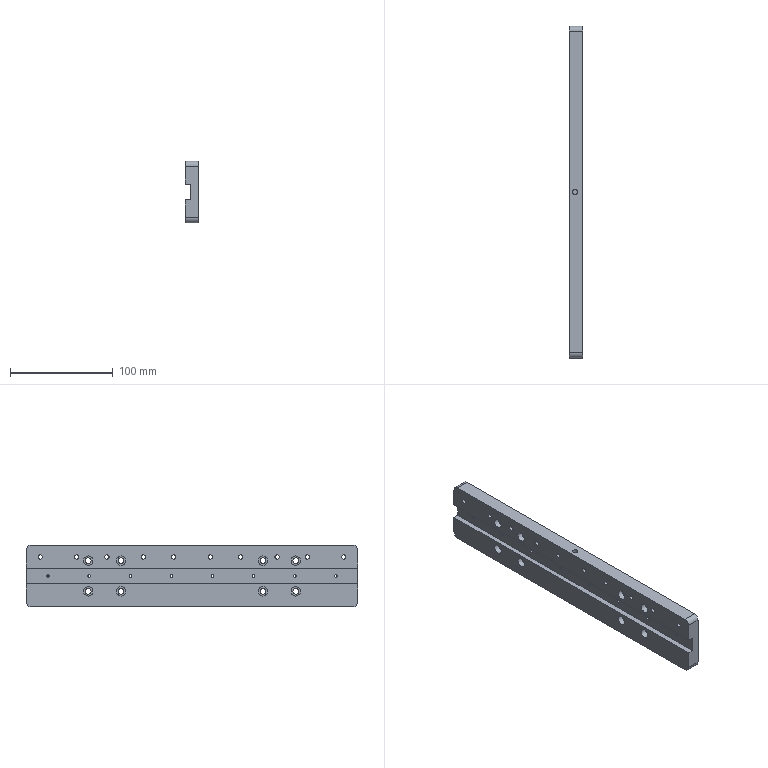CAM job | NX | 3+2 milling, drilling | part box 13 x 323 x 60 mm | stock box 15 x 328 x 65 mm
Tools:
number,name,description,diameter,corner_radius,flute_length,length,flutes
4,D4,平底铣刀-粗,4.0,0.0,25.0,75.0,2
9,D10,平底铣刀-粗,10.0,0.0,35.0,75.0,2
10,D10-J,平底铣刀-精,10.0,0.0,35.0,75.0,2
1,D80R0.8FLYCUTTER,圆鼻刀-粗,80.0,0.8,50.0,75.0,2
1,D80R0.8FLYCUTTER-J,圆鼻刀-精,80.0,0.8,50.0,75.0,2
2,D6CHAMFERMILL,倒角刀,6.0,0.0,3.0,25.0,2
20,M3X0.5,丝锥,2.5,0.0,35.0,50.0,2
22,M5X0.8,丝锥,4.2,0.0,35.0,50.0,2
14,ZT4.2,钻头,4.2,0.0,35.0,50.0,2
12,DRILL2.5,Twist Drill 2.5 mm,2.5,0.0,30.0,32.0,2
17,DRILL5.5,Twist Drill 5 mm,5.5,0.0,52.0,54.0,2
Operations:
program,operation,operation_type,tool,method,geometry_group,spindle_rpm,surface_speed,feed_per_tooth,feed_cut,feed_plunge,cut_length_mm,path_length_mm,cut_time_min,machine_time_min
B,FLOORFLYFACEROUGH_COPY,VolumeBased25DMillingOperation,D80R0.8FLYCUTTER,LAYERROUGH-DEPTHK-STEPG,W-B,2800.0,703.696,0.5357,3000.0,100.0,1724.918,3040.981,0.575,0.7066
B,FLOORFLYFACEFINISH_COPY,VolumeBased25DMillingOperation,D80R0.8FLYCUTTER-J,SIDEFINISH-DEPTHK-STEPG,W-B,4000.0,1005.28,0.125,1000.0,100.0,431.033,467.033,0.431,0.4346
B,DRILLCHAMFER_2,Operation,D6CHAMFERMILL,METHOD,W-B,8000.0,150.796,0.0625,1000.0,0.0,38.0,417.786,0.038,0.076
B,DRILLCHAMFER_3,Operation,D6CHAMFERMILL,METHOD,W-B,8000.0,150.796,0.0625,1000.0,0.0,57.0,477.741,0.057,0.0991
B,MILLCHAMFER_3,PlanarMilling,D6CHAMFERMILL,METHOD,W-B,8000.0,150.796,0.075,1200.0,100.0,142.357,802.749,0.1186,0.1847
B,C0.3CLOSEDCONTOURCHAMFER6X45L_COPY,PlanarMilling,D6CHAMFERMILL,CREEPCHAMFER-DEPTH0-STEPG,W-B,7000.0,131.0,0.1071,1500.0,100.0,775.048,811.048,0.5167,0.5203
A,TOPFACE,FaceMilling,D80R0.8FLYCUTTER,SIDEFINISH-DEPTHK-STEPG,W-A,5000.0,1256.637,0.1,1000.0,100.0,417.0,453.0,0.417,0.4206
A,PROFILEROUGH_2,VolumeBased25DMillingOperation,D10,METHOD,W-A,8000.0,251.327,0.3125,5000.0,80.0,15001.25,15052.85,3,3.005
A,FLOORWALLROUGH_1,VolumeBased25DMillingOperation,D10,METHOD,W-A,6000.0,113.0,0.2083,3500.0,100.0,6684.0,6806.058,1.91,1.922
A,SPOTDRILL-DEPTH0.8,Operation,D6CHAMFERMILL,NONE,W-A,8000.0,150.796,0.0312,500.0,90.0,46.8,751.771,0.0936,0.1641
A,THRUHOLE-M3TAPDRILL,Operation,DRILL2.5,NONE,W-A,3000.0,23.562,0.05,300.0,90.0,117.209,571.705,0.3907,0.4361
A,THRUHOLE-M5TAPDRILL,Operation,ZT4.2,NONE,W-A,3000.0,39.584,0.0583,350.0,90.0,212.618,769.874,0.6075,0.6632
A,COUNTERBORE-DRILL0SEG,Operation,DRILL5.5,NONE,W-A,2800.0,48.38,0.0357,200.0,90.0,141.219,651.539,0.7061,0.7571
A,CYLINDERROUGHD4_1,CylinderMilling,D4,NONE,W-A,8000.0,100.531,0.075,1200.0,100.0,3891.98,4621.98,3.243,3.316
A,CYLINDERFINISHD4_1,CylinderMilling,D4,FINISHSTEPDEPTHOFF,W-A,8000.0,100.531,0.0312,500.0,100.0,346.372,1028.372,0.6927,0.7609
A,SELECTBODYONLY,SurfaceContour,D6CHAMFERMILL,METHOD,W-A,8000.0,150.796,0.1875,3000.0,100.0,1461.87,2072.685,0.4873,0.5484
A,DRILLCHAMFER_1,Operation,D6CHAMFERMILL,METHOD,W-A,8000.0,150.796,0.0312,500.0,0.0,38.0,427.986,0.076,0.115
A,MILLCHAMFER_1,PlanarMilling,D6CHAMFERMILL,METHOD,W-A,8000.0,150.796,0.0312,500.0,100.0,180.203,873.214,0.3604,0.4297
A,MILLCHAMFER_2,PlanarMilling,D6CHAMFERMILL,NONE,W-A,8000.0,150.796,0.0312,500.0,100.0,296.875,901.107,0.5938,0.6542
A,THRUHOLE-TAPM3,Operation,M3X0.5,METHOD,W-A,800.0,6.283,0.0003,0.5,90.0,95.2,527.688,190.4,190.443
A,THRUHOLE-TAPM5,Operation,M5X0.8,METHOD,W-A,500.0,6.597,0.0008,0.8,90.0,175.0,694.638,218.75,218.802
A,BOTTOMSIDEFINISH_3,VolumeBased25DMillingOperation,D10-J,METHOD,W-A,6000.0,113.0,0.2083,1200.0,100.0,674.583,723.783,0.5622,0.5671
A,PROFILESEMIFINISH_2,VolumeBased25DMillingOperation,D10-J,METHOD,W-A,8000.0,251.327,0.0625,1000.0,100.0,793.828,859.028,0.7938,0.8003